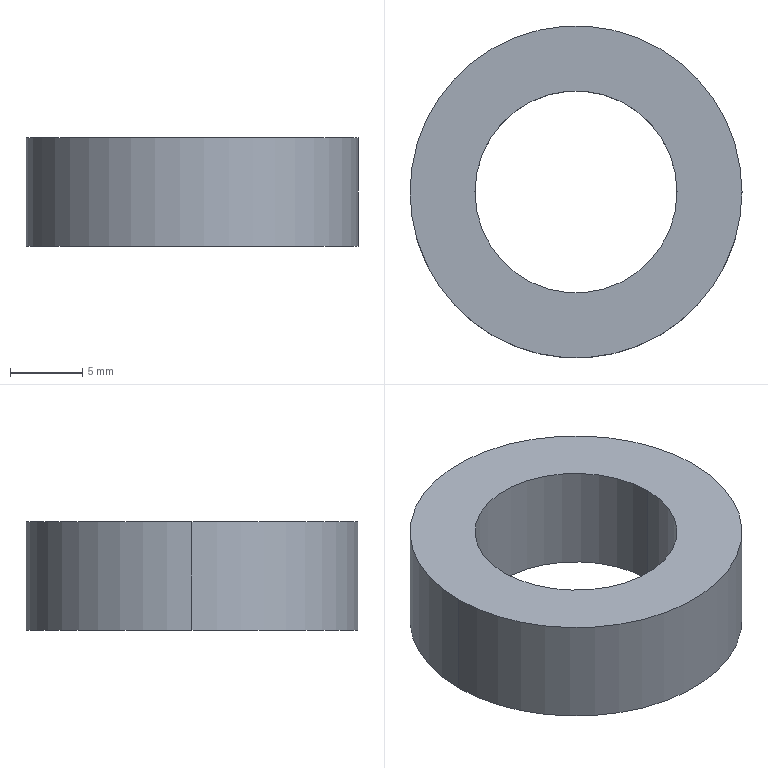Part | STEP file | Squeegee pressure rubber pad | 1 solid | 6 faces | box 23 x 23 x 7.5 mm | volume 1962 mm3 | cylinder 4 | plane 2 | commonest cylinder face diameters 14 x2 23 x2
STEP:
#1=CARTESIAN_POINT('',(-7.,0.,3.75));
#2=VERTEX_POINT('',#1);
#3=CARTESIAN_POINT('',(7.,0.,3.75));
#4=VERTEX_POINT('',#3);
#5=CARTESIAN_POINT('',(0.,0.,3.75));
#6=DIRECTION('',(0.,0.,1.));
#7=DIRECTION('',(1.,0.,0.));
#8=AXIS2_PLACEMENT_3D('',#5,#6,#7);
#9=CIRCLE('',#8,7.);
#10=EDGE_CURVE('',#2,#4,#9,.T.);
#11=ORIENTED_EDGE('',*,*,#10,.T.);
#12=CARTESIAN_POINT('',(7.,0.,-3.75));
#13=VERTEX_POINT('',#12);
#14=CARTESIAN_POINT('',(7.,0.,3.75));
#15=DIRECTION('',(0.,0.,-1.));
#16=VECTOR('',#15,1000.);
#17=LINE('',#14,#16);
#18=EDGE_CURVE('',#4,#13,#17,.T.);
#19=ORIENTED_EDGE('',*,*,#18,.T.);
#20=CARTESIAN_POINT('',(-7.,0.,-3.75));
#21=VERTEX_POINT('',#20);
#22=CARTESIAN_POINT('',(0.,0.,-3.75));
#23=DIRECTION('',(0.,0.,1.));
#24=DIRECTION('',(1.,0.,0.));
#25=AXIS2_PLACEMENT_3D('',#22,#23,#24);
#26=CIRCLE('',#25,7.);
#27=EDGE_CURVE('',#21,#13,#26,.T.);
#28=ORIENTED_EDGE('',*,*,#27,.F.);
#29=CARTESIAN_POINT('',(-7.,0.,3.75));
#30=DIRECTION('',(0.,0.,-1.));
#31=VECTOR('',#30,1000.);
#32=LINE('',#29,#31);
#33=EDGE_CURVE('',#2,#21,#32,.T.);
#34=ORIENTED_EDGE('',*,*,#33,.F.);
#35=EDGE_LOOP('',(#11,#19,#28,#34));
#36=FACE_OUTER_BOUND('',#35,.T.);
#37=CARTESIAN_POINT('',(0.,0.,3.75));
#38=DIRECTION('',(0.,0.,-1.));
#39=DIRECTION('',(-1.,0.,0.));
#40=AXIS2_PLACEMENT_3D('',#37,#38,#39);
#41=CYLINDRICAL_SURFACE('',#40,7.);
#42=ADVANCED_FACE('',(#36),#41,.F.);
#43=CARTESIAN_POINT('',(11.5,0.,3.75));
#44=VERTEX_POINT('',#43);
#45=CARTESIAN_POINT('',(-11.5,0.,3.75));
#46=VERTEX_POINT('',#45);
#47=CARTESIAN_POINT('',(0.,0.,3.75));
#48=DIRECTION('',(0.,0.,1.));
#49=DIRECTION('',(1.,0.,0.));
#50=AXIS2_PLACEMENT_3D('',#47,#48,#49);
#51=CIRCLE('',#50,11.5);
#52=EDGE_CURVE('',#44,#46,#51,.T.);
#53=ORIENTED_EDGE('',*,*,#52,.F.);
#54=CARTESIAN_POINT('',(11.5,0.,-3.75));
#55=VERTEX_POINT('',#54);
#56=CARTESIAN_POINT('',(11.5,0.,3.75));
#57=DIRECTION('',(0.,0.,-1.));
#58=VECTOR('',#57,1000.);
#59=LINE('',#56,#58);
#60=EDGE_CURVE('',#44,#55,#59,.T.);
#61=ORIENTED_EDGE('',*,*,#60,.T.);
#62=CARTESIAN_POINT('',(-11.5,0.,-3.75));
#63=VERTEX_POINT('',#62);
#64=CARTESIAN_POINT('',(0.,0.,-3.75));
#65=DIRECTION('',(0.,0.,1.));
#66=DIRECTION('',(1.,0.,0.));
#67=AXIS2_PLACEMENT_3D('',#64,#65,#66);
#68=CIRCLE('',#67,11.5);
#69=EDGE_CURVE('',#55,#63,#68,.T.);
#70=ORIENTED_EDGE('',*,*,#69,.T.);
#71=CARTESIAN_POINT('',(-11.5,0.,3.75));
#72=DIRECTION('',(0.,0.,-1.));
#73=VECTOR('',#72,1000.);
#74=LINE('',#71,#73);
#75=EDGE_CURVE('',#46,#63,#74,.T.);
#76=ORIENTED_EDGE('',*,*,#75,.F.);
#77=EDGE_LOOP('',(#53,#61,#70,#76));
#78=FACE_OUTER_BOUND('',#77,.T.);
#79=CARTESIAN_POINT('',(0.,0.,3.75));
#80=DIRECTION('',(0.,0.,-1.));
#81=DIRECTION('',(-1.,0.,0.));
#82=AXIS2_PLACEMENT_3D('',#79,#80,#81);
#83=CYLINDRICAL_SURFACE('',#82,11.5);
#84=ADVANCED_FACE('',(#78),#83,.T.);
#85=CARTESIAN_POINT('',(0.,0.,3.75));
#86=DIRECTION('',(0.,0.,1.));
#87=DIRECTION('',(1.,0.,0.));
#88=AXIS2_PLACEMENT_3D('',#85,#86,#87);
#89=CIRCLE('',#88,11.5);
#90=EDGE_CURVE('',#46,#44,#89,.T.);
#91=ORIENTED_EDGE('',*,*,#90,.T.);
#92=ORIENTED_EDGE('',*,*,#52,.T.);
#93=EDGE_LOOP('',(#91,#92));
#94=FACE_OUTER_BOUND('',#93,.T.);
#95=ORIENTED_EDGE('',*,*,#10,.F.);
#96=CARTESIAN_POINT('',(0.,0.,3.75));
#97=DIRECTION('',(0.,0.,1.));
#98=DIRECTION('',(1.,0.,0.));
#99=AXIS2_PLACEMENT_3D('',#96,#97,#98);
#100=CIRCLE('',#99,7.);
#101=EDGE_CURVE('',#4,#2,#100,.T.);
#102=ORIENTED_EDGE('',*,*,#101,.F.);
#103=EDGE_LOOP('',(#95,#102));
#104=FACE_BOUND('',#103,.T.);
#105=CARTESIAN_POINT('',(0.,0.,3.75));
#106=DIRECTION('',(0.,0.,1.));
#107=DIRECTION('',(1.,0.,0.));
#108=AXIS2_PLACEMENT_3D('',#105,#106,#107);
#109=PLANE('',#108);
#110=ADVANCED_FACE('',(#94,#104),#109,.T.);
#111=CARTESIAN_POINT('',(0.,0.,-3.75));
#112=DIRECTION('',(0.,0.,1.));
#113=DIRECTION('',(1.,0.,0.));
#114=AXIS2_PLACEMENT_3D('',#111,#112,#113);
#115=CIRCLE('',#114,11.5);
#116=EDGE_CURVE('',#63,#55,#115,.T.);
#117=ORIENTED_EDGE('',*,*,#116,.F.);
#118=ORIENTED_EDGE('',*,*,#69,.F.);
#119=EDGE_LOOP('',(#117,#118));
#120=FACE_OUTER_BOUND('',#119,.T.);
#121=ORIENTED_EDGE('',*,*,#27,.T.);
#122=CARTESIAN_POINT('',(0.,0.,-3.75));
#123=DIRECTION('',(0.,0.,1.));
#124=DIRECTION('',(1.,0.,0.));
#125=AXIS2_PLACEMENT_3D('',#122,#123,#124);
#126=CIRCLE('',#125,7.);
#127=EDGE_CURVE('',#13,#21,#126,.T.);
#128=ORIENTED_EDGE('',*,*,#127,.T.);
#129=EDGE_LOOP('',(#121,#128));
#130=FACE_BOUND('',#129,.T.);
#131=CARTESIAN_POINT('',(0.,0.,-3.75));
#132=DIRECTION('',(0.,0.,1.));
#133=DIRECTION('',(1.,0.,0.));
#134=AXIS2_PLACEMENT_3D('',#131,#132,#133);
#135=PLANE('',#134);
#136=ADVANCED_FACE('',(#120,#130),#135,.F.);
#137=ORIENTED_EDGE('',*,*,#60,.F.);
#138=ORIENTED_EDGE('',*,*,#90,.F.);
#139=ORIENTED_EDGE('',*,*,#75,.T.);
#140=ORIENTED_EDGE('',*,*,#116,.T.);
#141=EDGE_LOOP('',(#137,#138,#139,#140));
#142=FACE_OUTER_BOUND('',#141,.T.);
#143=CARTESIAN_POINT('',(0.,0.,3.75));
#144=DIRECTION('',(0.,0.,-1.));
#145=DIRECTION('',(-1.,0.,0.));
#146=AXIS2_PLACEMENT_3D('',#143,#144,#145);
#147=CYLINDRICAL_SURFACE('',#146,11.5);
#148=ADVANCED_FACE('',(#142),#147,.T.);
#149=ORIENTED_EDGE('',*,*,#18,.F.);
#150=ORIENTED_EDGE('',*,*,#101,.T.);
#151=ORIENTED_EDGE('',*,*,#33,.T.);
#152=ORIENTED_EDGE('',*,*,#127,.F.);
#153=EDGE_LOOP('',(#149,#150,#151,#152));
#154=FACE_OUTER_BOUND('',#153,.T.);
#155=CARTESIAN_POINT('',(0.,0.,3.75));
#156=DIRECTION('',(0.,0.,-1.));
#157=DIRECTION('',(-1.,0.,0.));
#158=AXIS2_PLACEMENT_3D('',#155,#156,#157);
#159=CYLINDRICAL_SURFACE('',#158,7.);
#160=ADVANCED_FACE('',(#154),#159,.F.);
#161=CLOSED_SHELL('',(#42,#84,#110,#136,#148,#160));
#162=MANIFOLD_SOLID_BREP('',#161);
#163=CARTESIAN_POINT('',(0.,0.,0.));
#164=DIRECTION('',(0.,0.,1.));
#165=DIRECTION('',(1.,0.,0.));
#166=AXIS2_PLACEMENT_3D('',#163,#164,#165);
#167=(LENGTH_UNIT()NAMED_UNIT(*)SI_UNIT(.MILLI.,.METRE.));
#168=UNCERTAINTY_MEASURE_WITH_UNIT(LENGTH_MEASURE(0.00001),#167,'','');
#169=(NAMED_UNIT(*)PLANE_ANGLE_UNIT()SI_UNIT($,.RADIAN.));
#170=(NAMED_UNIT(*)SI_UNIT($,.STERADIAN.)SOLID_ANGLE_UNIT());
#171=(GEOMETRIC_REPRESENTATION_CONTEXT(3)GLOBAL_UNCERTAINTY_ASSIGNED_CONTEXT((#168))GLOBAL_UNIT_ASSIGNED_CONTEXT((#167,#169,#170))REPRESENTATION_CONTEXT('',''));
#172=ADVANCED_BREP_SHAPE_REPRESENTATION('',(#162,#166),#171);